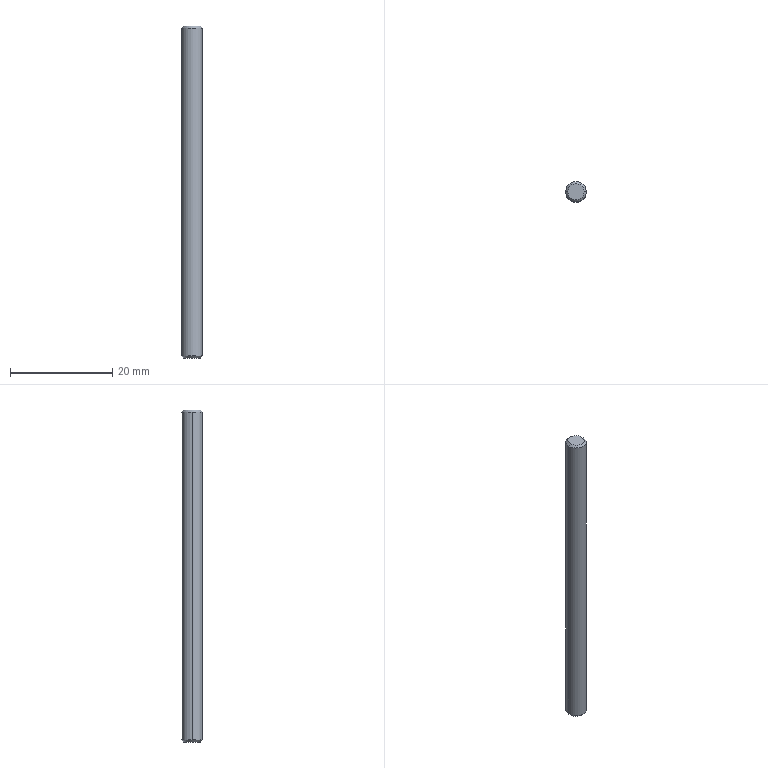Part | NX | features BREP 1 | 1 solid | 8 faces | box 4 x 4 x 65 mm | volume 814.938 mm3 | cone 4 | cylinder 2 | plane 2 | commonest cylinder face diameters 4 x2
STEP:
#1=CARTESIAN_POINT('',(-1.6,0.,0.));
#2=VERTEX_POINT('',#1);
#3=CARTESIAN_POINT('',(1.6,0.,0.));
#4=VERTEX_POINT('',#3);
#5=CARTESIAN_POINT('',(0.,0.,0.));
#6=DIRECTION('',(0.,0.,-1.));
#7=DIRECTION('',(-1.,0.,0.));
#8=AXIS2_PLACEMENT_3D('',#5,#6,#7);
#9=CIRCLE('',#8,1.6);
#10=EDGE_CURVE('',#2,#4,#9,.T.);
#11=ORIENTED_EDGE('',*,*,#10,.T.);
#12=CARTESIAN_POINT('',(2.,0.,-0.4));
#13=VERTEX_POINT('',#12);
#14=CARTESIAN_POINT('',(1.6,0.,0.));
#15=DIRECTION('',(0.7071,0.,-0.7071));
#16=VECTOR('',#15,1000.);
#17=LINE('',#14,#16);
#18=EDGE_CURVE('',#4,#13,#17,.T.);
#19=ORIENTED_EDGE('',*,*,#18,.T.);
#20=CARTESIAN_POINT('',(-2.,0.,-0.4));
#21=VERTEX_POINT('',#20);
#22=CARTESIAN_POINT('',(0.,0.,-0.4));
#23=DIRECTION('',(0.,0.,-1.));
#24=DIRECTION('',(-1.,0.,0.));
#25=AXIS2_PLACEMENT_3D('',#22,#23,#24);
#26=CIRCLE('',#25,2.);
#27=EDGE_CURVE('',#21,#13,#26,.T.);
#28=ORIENTED_EDGE('',*,*,#27,.F.);
#29=CARTESIAN_POINT('',(-1.6,0.,0.));
#30=DIRECTION('',(-0.7071,0.,-0.7071));
#31=VECTOR('',#30,1000.);
#32=LINE('',#29,#31);
#33=EDGE_CURVE('',#2,#21,#32,.T.);
#34=ORIENTED_EDGE('',*,*,#33,.F.);
#35=EDGE_LOOP('',(#11,#19,#28,#34));
#36=FACE_BOUND('',#35,.T.);
#37=CARTESIAN_POINT('',(0.,0.,0.));
#38=DIRECTION('',(0.,0.,-1.));
#39=DIRECTION('',(-1.,0.,0.));
#40=AXIS2_PLACEMENT_3D('',#37,#38,#39);
#41=CONICAL_SURFACE('',#40,1.6,0.7854);
#42=ADVANCED_FACE('',(#36),#41,.T.);
#43=ORIENTED_EDGE('',*,*,#27,.T.);
#44=CARTESIAN_POINT('',(2.,0.,-64.6));
#45=VERTEX_POINT('',#44);
#46=CARTESIAN_POINT('',(2.,0.,0.));
#47=DIRECTION('',(0.,0.,-1.));
#48=VECTOR('',#47,1000.);
#49=LINE('',#46,#48);
#50=EDGE_CURVE('',#13,#45,#49,.T.);
#51=ORIENTED_EDGE('',*,*,#50,.T.);
#52=CARTESIAN_POINT('',(-2.,0.,-64.6));
#53=VERTEX_POINT('',#52);
#54=CARTESIAN_POINT('',(0.,0.,-64.6));
#55=DIRECTION('',(0.,0.,-1.));
#56=DIRECTION('',(-1.,0.,0.));
#57=AXIS2_PLACEMENT_3D('',#54,#55,#56);
#58=CIRCLE('',#57,2.);
#59=EDGE_CURVE('',#53,#45,#58,.T.);
#60=ORIENTED_EDGE('',*,*,#59,.F.);
#61=CARTESIAN_POINT('',(-2.,0.,0.));
#62=DIRECTION('',(0.,0.,-1.));
#63=VECTOR('',#62,1000.);
#64=LINE('',#61,#63);
#65=EDGE_CURVE('',#21,#53,#64,.T.);
#66=ORIENTED_EDGE('',*,*,#65,.F.);
#67=EDGE_LOOP('',(#43,#51,#60,#66));
#68=FACE_BOUND('',#67,.T.);
#69=CARTESIAN_POINT('',(0.,0.,0.));
#70=DIRECTION('',(0.,0.,-1.));
#71=DIRECTION('',(-1.,0.,0.));
#72=AXIS2_PLACEMENT_3D('',#69,#70,#71);
#73=CYLINDRICAL_SURFACE('',#72,2.);
#74=ADVANCED_FACE('',(#68),#73,.T.);
#75=CARTESIAN_POINT('',(-1.6,0.,-65.));
#76=VERTEX_POINT('',#75);
#77=CARTESIAN_POINT('',(1.6,0.,-65.));
#78=VERTEX_POINT('',#77);
#79=CARTESIAN_POINT('',(0.,0.,-65.));
#80=DIRECTION('',(0.,0.,-1.));
#81=DIRECTION('',(-1.,0.,0.));
#82=AXIS2_PLACEMENT_3D('',#79,#80,#81);
#83=CIRCLE('',#82,1.6);
#84=EDGE_CURVE('',#76,#78,#83,.T.);
#85=ORIENTED_EDGE('',*,*,#84,.F.);
#86=CARTESIAN_POINT('',(-2.,0.,-64.6));
#87=DIRECTION('',(-0.7071,0.,0.7071));
#88=VECTOR('',#87,1000.);
#89=LINE('',#86,#88);
#90=EDGE_CURVE('',#53,#76,#89,.F.);
#91=ORIENTED_EDGE('',*,*,#90,.F.);
#92=ORIENTED_EDGE('',*,*,#59,.T.);
#93=CARTESIAN_POINT('',(2.,0.,-64.6));
#94=DIRECTION('',(0.7071,0.,0.7071));
#95=VECTOR('',#94,1000.);
#96=LINE('',#93,#95);
#97=EDGE_CURVE('',#45,#78,#96,.F.);
#98=ORIENTED_EDGE('',*,*,#97,.T.);
#99=EDGE_LOOP('',(#85,#91,#92,#98));
#100=FACE_BOUND('',#99,.T.);
#101=CARTESIAN_POINT('',(0.,0.,-64.6));
#102=DIRECTION('',(0.,0.,1.));
#103=DIRECTION('',(1.,0.,0.));
#104=AXIS2_PLACEMENT_3D('',#101,#102,#103);
#105=CONICAL_SURFACE('',#104,2.,0.7854);
#106=ADVANCED_FACE('',(#100),#105,.T.);
#107=CARTESIAN_POINT('',(0.,0.,-65.));
#108=DIRECTION('',(0.,0.,-1.));
#109=DIRECTION('',(-1.,0.,0.));
#110=AXIS2_PLACEMENT_3D('',#107,#108,#109);
#111=CIRCLE('',#110,1.6);
#112=EDGE_CURVE('',#78,#76,#111,.T.);
#113=ORIENTED_EDGE('',*,*,#112,.T.);
#114=ORIENTED_EDGE('',*,*,#84,.T.);
#115=EDGE_LOOP('',(#113,#114));
#116=FACE_BOUND('',#115,.T.);
#117=CARTESIAN_POINT('',(0.,0.,-65.));
#118=DIRECTION('',(0.,0.,1.));
#119=DIRECTION('',(1.,0.,0.));
#120=AXIS2_PLACEMENT_3D('',#117,#118,#119);
#121=PLANE('',#120);
#122=ADVANCED_FACE('',(#116),#121,.F.);
#123=ORIENTED_EDGE('',*,*,#90,.T.);
#124=ORIENTED_EDGE('',*,*,#112,.F.);
#125=ORIENTED_EDGE('',*,*,#97,.F.);
#126=CARTESIAN_POINT('',(0.,0.,-64.6));
#127=DIRECTION('',(0.,0.,-1.));
#128=DIRECTION('',(-1.,0.,0.));
#129=AXIS2_PLACEMENT_3D('',#126,#127,#128);
#130=CIRCLE('',#129,2.);
#131=EDGE_CURVE('',#45,#53,#130,.T.);
#132=ORIENTED_EDGE('',*,*,#131,.T.);
#133=EDGE_LOOP('',(#123,#124,#125,#132));
#134=FACE_BOUND('',#133,.T.);
#135=CARTESIAN_POINT('',(0.,0.,-64.6));
#136=DIRECTION('',(0.,0.,1.));
#137=DIRECTION('',(1.,0.,0.));
#138=AXIS2_PLACEMENT_3D('',#135,#136,#137);
#139=CONICAL_SURFACE('',#138,2.,0.7854);
#140=ADVANCED_FACE('',(#134),#139,.T.);
#141=ORIENTED_EDGE('',*,*,#50,.F.);
#142=CARTESIAN_POINT('',(0.,0.,-0.4));
#143=DIRECTION('',(0.,0.,-1.));
#144=DIRECTION('',(-1.,0.,0.));
#145=AXIS2_PLACEMENT_3D('',#142,#143,#144);
#146=CIRCLE('',#145,2.);
#147=EDGE_CURVE('',#13,#21,#146,.T.);
#148=ORIENTED_EDGE('',*,*,#147,.T.);
#149=ORIENTED_EDGE('',*,*,#65,.T.);
#150=ORIENTED_EDGE('',*,*,#131,.F.);
#151=EDGE_LOOP('',(#141,#148,#149,#150));
#152=FACE_BOUND('',#151,.T.);
#153=CARTESIAN_POINT('',(0.,0.,0.));
#154=DIRECTION('',(0.,0.,-1.));
#155=DIRECTION('',(-1.,0.,0.));
#156=AXIS2_PLACEMENT_3D('',#153,#154,#155);
#157=CYLINDRICAL_SURFACE('',#156,2.);
#158=ADVANCED_FACE('',(#152),#157,.T.);
#159=ORIENTED_EDGE('',*,*,#18,.F.);
#160=CARTESIAN_POINT('',(0.,0.,0.));
#161=DIRECTION('',(0.,0.,-1.));
#162=DIRECTION('',(-1.,0.,0.));
#163=AXIS2_PLACEMENT_3D('',#160,#161,#162);
#164=CIRCLE('',#163,1.6);
#165=EDGE_CURVE('',#4,#2,#164,.T.);
#166=ORIENTED_EDGE('',*,*,#165,.T.);
#167=ORIENTED_EDGE('',*,*,#33,.T.);
#168=ORIENTED_EDGE('',*,*,#147,.F.);
#169=EDGE_LOOP('',(#159,#166,#167,#168));
#170=FACE_BOUND('',#169,.T.);
#171=CARTESIAN_POINT('',(0.,0.,0.));
#172=DIRECTION('',(0.,0.,-1.));
#173=DIRECTION('',(-1.,0.,0.));
#174=AXIS2_PLACEMENT_3D('',#171,#172,#173);
#175=CONICAL_SURFACE('',#174,1.6,0.7854);
#176=ADVANCED_FACE('',(#170),#175,.T.);
#177=ORIENTED_EDGE('',*,*,#10,.F.);
#178=ORIENTED_EDGE('',*,*,#165,.F.);
#179=EDGE_LOOP('',(#177,#178));
#180=FACE_BOUND('',#179,.T.);
#181=CARTESIAN_POINT('',(1.6,0.,0.));
#182=DIRECTION('',(0.,0.,-1.));
#183=DIRECTION('',(0.,-1.,0.));
#184=AXIS2_PLACEMENT_3D('',#181,#182,#183);
#185=PLANE('',#184);
#186=ADVANCED_FACE('',(#180),#185,.F.);
#187=CLOSED_SHELL('',(#42,#74,#106,#122,#140,#158,#176,#186));
#188=MANIFOLD_SOLID_BREP('',#187);
#189=(LENGTH_UNIT()NAMED_UNIT(*)SI_UNIT(.MILLI.,.METRE.));
#190=UNCERTAINTY_MEASURE_WITH_UNIT(LENGTH_MEASURE(0.00001),#189,'','');
#191=(NAMED_UNIT(*)PLANE_ANGLE_UNIT()SI_UNIT($,.RADIAN.));
#192=(NAMED_UNIT(*)SI_UNIT($,.STERADIAN.)SOLID_ANGLE_UNIT());
#193=(GEOMETRIC_REPRESENTATION_CONTEXT(3)GLOBAL_UNCERTAINTY_ASSIGNED_CONTEXT((#190))GLOBAL_UNIT_ASSIGNED_CONTEXT((#189,#191,#192))REPRESENTATION_CONTEXT('',''));
#194=ADVANCED_BREP_SHAPE_REPRESENTATION('',(#188),#193);